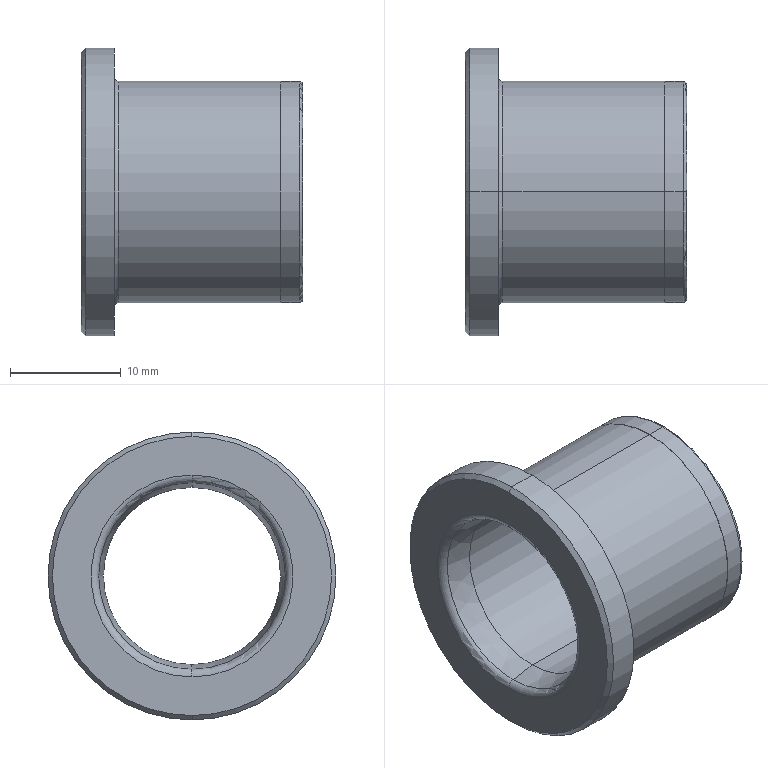Part | SolidWorks | features Revolution 1 | 1 solid | 24 faces | box 20 x 26 x 26 mm | volume 2854 mm3 | cylinder 8 | torus 8 | cone 4 | plane 4 | commonest cylinder face diameters 16 x2 19.96 x2 20 x2 26 x2
STEP:
#1=CARTESIAN_POINT('',(3.,0.,13.));
#2=VERTEX_POINT('',#1);
#3=CARTESIAN_POINT('',(3.,0.,-13.));
#4=VERTEX_POINT('',#3);
#5=CARTESIAN_POINT('',(3.,0.,0.));
#6=DIRECTION('',(-1.,0.,0.));
#7=DIRECTION('',(0.,0.,1.));
#8=AXIS2_PLACEMENT_3D('',#5,#6,#7);
#9=CIRCLE('',#8,13.);
#10=EDGE_CURVE('',#2,#4,#9,.T.);
#11=ORIENTED_EDGE('',*,*,#10,.T.);
#12=CARTESIAN_POINT('',(0.4,0.,-13.));
#13=VERTEX_POINT('',#12);
#14=CARTESIAN_POINT('',(20.,0.,-13.));
#15=DIRECTION('',(-1.,0.,0.));
#16=VECTOR('',#15,1000.);
#17=LINE('',#14,#16);
#18=EDGE_CURVE('',#4,#13,#17,.T.);
#19=ORIENTED_EDGE('',*,*,#18,.T.);
#20=CARTESIAN_POINT('',(0.4,0.,13.));
#21=VERTEX_POINT('',#20);
#22=CARTESIAN_POINT('',(0.4,0.,0.));
#23=DIRECTION('',(-1.,0.,0.));
#24=DIRECTION('',(0.,0.,1.));
#25=AXIS2_PLACEMENT_3D('',#22,#23,#24);
#26=CIRCLE('',#25,13.);
#27=EDGE_CURVE('',#21,#13,#26,.T.);
#28=ORIENTED_EDGE('',*,*,#27,.F.);
#29=CARTESIAN_POINT('',(20.,0.,13.));
#30=DIRECTION('',(-1.,0.,0.));
#31=VECTOR('',#30,1000.);
#32=LINE('',#29,#31);
#33=EDGE_CURVE('',#2,#21,#32,.T.);
#34=ORIENTED_EDGE('',*,*,#33,.F.);
#35=EDGE_LOOP('',(#11,#19,#28,#34));
#36=FACE_OUTER_BOUND('',#35,.T.);
#37=CARTESIAN_POINT('',(20.,0.,0.));
#38=DIRECTION('',(-1.,0.,0.));
#39=DIRECTION('',(0.,0.,1.));
#40=AXIS2_PLACEMENT_3D('',#37,#38,#39);
#41=CYLINDRICAL_SURFACE('',#40,13.);
#42=ADVANCED_FACE('',(#36),#41,.T.);
#43=CARTESIAN_POINT('',(3.,0.,-10.4));
#44=VERTEX_POINT('',#43);
#45=CARTESIAN_POINT('',(3.,0.,10.4));
#46=VERTEX_POINT('',#45);
#47=CARTESIAN_POINT('',(3.,0.,0.));
#48=DIRECTION('',(-1.,0.,0.));
#49=DIRECTION('',(0.,0.,1.));
#50=AXIS2_PLACEMENT_3D('',#47,#48,#49);
#51=CIRCLE('',#50,10.4);
#52=EDGE_CURVE('',#44,#46,#51,.T.);
#53=ORIENTED_EDGE('',*,*,#52,.F.);
#54=CARTESIAN_POINT('',(3.4,0.,-10.));
#55=VERTEX_POINT('',#54);
#56=CARTESIAN_POINT('',(3.4,0.,-10.4));
#57=DIRECTION('',(0.,1.,0.));
#58=DIRECTION('',(0.,0.,1.));
#59=AXIS2_PLACEMENT_3D('',#56,#57,#58);
#60=CIRCLE('',#59,0.4);
#61=EDGE_CURVE('',#44,#55,#60,.T.);
#62=ORIENTED_EDGE('',*,*,#61,.T.);
#63=CARTESIAN_POINT('',(3.4,0.,10.));
#64=VERTEX_POINT('',#63);
#65=CARTESIAN_POINT('',(3.4,0.,0.));
#66=DIRECTION('',(-1.,0.,0.));
#67=DIRECTION('',(0.,0.,1.));
#68=AXIS2_PLACEMENT_3D('',#65,#66,#67);
#69=CIRCLE('',#68,10.);
#70=EDGE_CURVE('',#55,#64,#69,.T.);
#71=ORIENTED_EDGE('',*,*,#70,.T.);
#72=CARTESIAN_POINT('',(3.4,0.,10.4));
#73=DIRECTION('',(0.,-1.,0.));
#74=DIRECTION('',(0.,0.,-1.));
#75=AXIS2_PLACEMENT_3D('',#72,#73,#74);
#76=CIRCLE('',#75,0.4);
#77=EDGE_CURVE('',#46,#64,#76,.T.);
#78=ORIENTED_EDGE('',*,*,#77,.F.);
#79=EDGE_LOOP('',(#53,#62,#71,#78));
#80=FACE_OUTER_BOUND('',#79,.T.);
#81=CARTESIAN_POINT('',(3.4,0.,0.));
#82=DIRECTION('',(-1.,0.,0.));
#83=DIRECTION('',(0.,0.,1.));
#84=AXIS2_PLACEMENT_3D('',#81,#82,#83);
#85=TOROIDAL_SURFACE('',#84,10.4,0.4);
#86=ADVANCED_FACE('',(#80),#85,.F.);
#87=CARTESIAN_POINT('',(18.,0.,10.));
#88=VERTEX_POINT('',#87);
#89=CARTESIAN_POINT('',(18.,0.,-10.));
#90=VERTEX_POINT('',#89);
#91=CARTESIAN_POINT('',(18.,0.,0.));
#92=DIRECTION('',(-1.,0.,0.));
#93=DIRECTION('',(0.,0.,1.));
#94=AXIS2_PLACEMENT_3D('',#91,#92,#93);
#95=CIRCLE('',#94,10.);
#96=EDGE_CURVE('',#88,#90,#95,.T.);
#97=ORIENTED_EDGE('',*,*,#96,.T.);
#98=CARTESIAN_POINT('',(20.,0.,-10.));
#99=DIRECTION('',(-1.,0.,0.));
#100=VECTOR('',#99,1000.);
#101=LINE('',#98,#100);
#102=EDGE_CURVE('',#90,#55,#101,.T.);
#103=ORIENTED_EDGE('',*,*,#102,.T.);
#104=CARTESIAN_POINT('',(3.4,0.,0.));
#105=DIRECTION('',(-1.,0.,0.));
#106=DIRECTION('',(0.,0.,1.));
#107=AXIS2_PLACEMENT_3D('',#104,#105,#106);
#108=CIRCLE('',#107,10.);
#109=EDGE_CURVE('',#64,#55,#108,.T.);
#110=ORIENTED_EDGE('',*,*,#109,.F.);
#111=CARTESIAN_POINT('',(20.,0.,10.));
#112=DIRECTION('',(-1.,0.,0.));
#113=VECTOR('',#112,1000.);
#114=LINE('',#111,#113);
#115=EDGE_CURVE('',#88,#64,#114,.T.);
#116=ORIENTED_EDGE('',*,*,#115,.F.);
#117=EDGE_LOOP('',(#97,#103,#110,#116));
#118=FACE_OUTER_BOUND('',#117,.T.);
#119=CARTESIAN_POINT('',(20.,0.,0.));
#120=DIRECTION('',(-1.,0.,0.));
#121=DIRECTION('',(0.,0.,1.));
#122=AXIS2_PLACEMENT_3D('',#119,#120,#121);
#123=CYLINDRICAL_SURFACE('',#122,10.);
#124=ADVANCED_FACE('',(#118),#123,.T.);
#125=CARTESIAN_POINT('',(19.7,0.,9.98));
#126=VERTEX_POINT('',#125);
#127=CARTESIAN_POINT('',(19.7,0.,-9.98));
#128=VERTEX_POINT('',#127);
#129=CARTESIAN_POINT('',(19.7,0.,0.));
#130=DIRECTION('',(-1.,0.,0.));
#131=DIRECTION('',(0.,0.,1.));
#132=AXIS2_PLACEMENT_3D('',#129,#130,#131);
#133=CIRCLE('',#132,9.98);
#134=EDGE_CURVE('',#126,#128,#133,.T.);
#135=ORIENTED_EDGE('',*,*,#134,.T.);
#136=CARTESIAN_POINT('',(18.,0.,-9.98));
#137=VERTEX_POINT('',#136);
#138=CARTESIAN_POINT('',(20.,0.,-9.98));
#139=DIRECTION('',(-1.,0.,0.));
#140=VECTOR('',#139,1000.);
#141=LINE('',#138,#140);
#142=EDGE_CURVE('',#128,#137,#141,.T.);
#143=ORIENTED_EDGE('',*,*,#142,.T.);
#144=CARTESIAN_POINT('',(18.,0.,9.98));
#145=VERTEX_POINT('',#144);
#146=CARTESIAN_POINT('',(18.,0.,0.));
#147=DIRECTION('',(-1.,0.,0.));
#148=DIRECTION('',(0.,0.,1.));
#149=AXIS2_PLACEMENT_3D('',#146,#147,#148);
#150=CIRCLE('',#149,9.98);
#151=EDGE_CURVE('',#145,#137,#150,.T.);
#152=ORIENTED_EDGE('',*,*,#151,.F.);
#153=CARTESIAN_POINT('',(20.,0.,9.98));
#154=DIRECTION('',(-1.,0.,0.));
#155=VECTOR('',#154,1000.);
#156=LINE('',#153,#155);
#157=EDGE_CURVE('',#126,#145,#156,.T.);
#158=ORIENTED_EDGE('',*,*,#157,.F.);
#159=EDGE_LOOP('',(#135,#143,#152,#158));
#160=FACE_OUTER_BOUND('',#159,.T.);
#161=CARTESIAN_POINT('',(20.,0.,0.));
#162=DIRECTION('',(-1.,0.,0.));
#163=DIRECTION('',(0.,0.,1.));
#164=AXIS2_PLACEMENT_3D('',#161,#162,#163);
#165=CYLINDRICAL_SURFACE('',#164,9.98);
#166=ADVANCED_FACE('',(#160),#165,.T.);
#167=CARTESIAN_POINT('',(20.,0.,9.68));
#168=VERTEX_POINT('',#167);
#169=CARTESIAN_POINT('',(20.,0.,-9.68));
#170=VERTEX_POINT('',#169);
#171=CARTESIAN_POINT('',(20.,0.,0.));
#172=DIRECTION('',(-1.,0.,0.));
#173=DIRECTION('',(0.,0.,1.));
#174=AXIS2_PLACEMENT_3D('',#171,#172,#173);
#175=CIRCLE('',#174,9.68);
#176=EDGE_CURVE('',#168,#170,#175,.T.);
#177=ORIENTED_EDGE('',*,*,#176,.T.);
#178=CARTESIAN_POINT('',(19.7,0.,-9.68));
#179=DIRECTION('',(0.,1.,0.));
#180=DIRECTION('',(0.,0.,1.));
#181=AXIS2_PLACEMENT_3D('',#178,#179,#180);
#182=CIRCLE('',#181,0.3);
#183=EDGE_CURVE('',#170,#128,#182,.T.);
#184=ORIENTED_EDGE('',*,*,#183,.T.);
#185=ORIENTED_EDGE('',*,*,#134,.F.);
#186=CARTESIAN_POINT('',(19.7,0.,9.68));
#187=DIRECTION('',(0.,-1.,0.));
#188=DIRECTION('',(0.,0.,-1.));
#189=AXIS2_PLACEMENT_3D('',#186,#187,#188);
#190=CIRCLE('',#189,0.3);
#191=EDGE_CURVE('',#168,#126,#190,.T.);
#192=ORIENTED_EDGE('',*,*,#191,.F.);
#193=EDGE_LOOP('',(#177,#184,#185,#192));
#194=FACE_OUTER_BOUND('',#193,.T.);
#195=CARTESIAN_POINT('',(19.7,0.,0.));
#196=DIRECTION('',(-1.,0.,0.));
#197=DIRECTION('',(0.,0.,1.));
#198=AXIS2_PLACEMENT_3D('',#195,#196,#197);
#199=TOROIDAL_SURFACE('',#198,9.68,0.3);
#200=ADVANCED_FACE('',(#194),#199,.T.);
#201=CARTESIAN_POINT('',(19.3,0.,8.));
#202=VERTEX_POINT('',#201);
#203=CARTESIAN_POINT('',(19.3,0.,-8.));
#204=VERTEX_POINT('',#203);
#205=CARTESIAN_POINT('',(19.3,0.,0.));
#206=DIRECTION('',(-1.,0.,0.));
#207=DIRECTION('',(0.,0.,1.));
#208=AXIS2_PLACEMENT_3D('',#205,#206,#207);
#209=CIRCLE('',#208,8.);
#210=EDGE_CURVE('',#202,#204,#209,.T.);
#211=ORIENTED_EDGE('',*,*,#210,.T.);
#212=CARTESIAN_POINT('',(20.,0.,-8.7));
#213=VERTEX_POINT('',#212);
#214=CARTESIAN_POINT('',(19.3,0.,-8.7));
#215=DIRECTION('',(0.,1.,0.));
#216=DIRECTION('',(0.,0.,1.));
#217=AXIS2_PLACEMENT_3D('',#214,#215,#216);
#218=CIRCLE('',#217,0.7);
#219=EDGE_CURVE('',#204,#213,#218,.T.);
#220=ORIENTED_EDGE('',*,*,#219,.T.);
#221=CARTESIAN_POINT('',(20.,0.,8.7));
#222=VERTEX_POINT('',#221);
#223=CARTESIAN_POINT('',(20.,0.,0.));
#224=DIRECTION('',(-1.,0.,0.));
#225=DIRECTION('',(0.,0.,1.));
#226=AXIS2_PLACEMENT_3D('',#223,#224,#225);
#227=CIRCLE('',#226,8.7);
#228=EDGE_CURVE('',#222,#213,#227,.T.);
#229=ORIENTED_EDGE('',*,*,#228,.F.);
#230=CARTESIAN_POINT('',(19.3,0.,8.7));
#231=DIRECTION('',(0.,-1.,0.));
#232=DIRECTION('',(0.,0.,-1.));
#233=AXIS2_PLACEMENT_3D('',#230,#231,#232);
#234=CIRCLE('',#233,0.7);
#235=EDGE_CURVE('',#202,#222,#234,.T.);
#236=ORIENTED_EDGE('',*,*,#235,.F.);
#237=EDGE_LOOP('',(#211,#220,#229,#236));
#238=FACE_OUTER_BOUND('',#237,.T.);
#239=CARTESIAN_POINT('',(19.3,0.,0.));
#240=DIRECTION('',(-1.,0.,0.));
#241=DIRECTION('',(0.,0.,1.));
#242=AXIS2_PLACEMENT_3D('',#239,#240,#241);
#243=TOROIDAL_SURFACE('',#242,8.7,0.7);
#244=ADVANCED_FACE('',(#238),#243,.T.);
#245=CARTESIAN_POINT('',(19.3,0.,0.));
#246=DIRECTION('',(-1.,0.,0.));
#247=DIRECTION('',(0.,0.,1.));
#248=AXIS2_PLACEMENT_3D('',#245,#246,#247);
#249=CIRCLE('',#248,8.);
#250=EDGE_CURVE('',#204,#202,#249,.T.);
#251=ORIENTED_EDGE('',*,*,#250,.F.);
#252=CARTESIAN_POINT('',(3.,0.,-8.));
#253=VERTEX_POINT('',#252);
#254=CARTESIAN_POINT('',(20.,0.,-8.));
#255=DIRECTION('',(-1.,0.,0.));
#256=VECTOR('',#255,1000.);
#257=LINE('',#254,#256);
#258=EDGE_CURVE('',#204,#253,#257,.T.);
#259=ORIENTED_EDGE('',*,*,#258,.T.);
#260=CARTESIAN_POINT('',(3.,0.,8.));
#261=VERTEX_POINT('',#260);
#262=CARTESIAN_POINT('',(3.,0.,0.));
#263=DIRECTION('',(-1.,0.,0.));
#264=DIRECTION('',(0.,0.,1.));
#265=AXIS2_PLACEMENT_3D('',#262,#263,#264);
#266=CIRCLE('',#265,8.);
#267=EDGE_CURVE('',#253,#261,#266,.T.);
#268=ORIENTED_EDGE('',*,*,#267,.T.);
#269=CARTESIAN_POINT('',(20.,0.,8.));
#270=DIRECTION('',(-1.,0.,0.));
#271=VECTOR('',#270,1000.);
#272=LINE('',#269,#271);
#273=EDGE_CURVE('',#202,#261,#272,.T.);
#274=ORIENTED_EDGE('',*,*,#273,.F.);
#275=EDGE_LOOP('',(#251,#259,#268,#274));
#276=FACE_OUTER_BOUND('',#275,.T.);
#277=CARTESIAN_POINT('',(20.,0.,0.));
#278=DIRECTION('',(-1.,0.,0.));
#279=DIRECTION('',(0.,0.,1.));
#280=AXIS2_PLACEMENT_3D('',#277,#278,#279);
#281=CYLINDRICAL_SURFACE('',#280,8.);
#282=ADVANCED_FACE('',(#276),#281,.F.);
#283=ORIENTED_EDGE('',*,*,#267,.F.);
#284=CARTESIAN_POINT('',(0.5784,0.,-8.427));
#285=VERTEX_POINT('',#284);
#286=CARTESIAN_POINT('',(0.5784,0.,-8.427));
#287=DIRECTION('',(-0.9848,0.,-0.1736));
#288=VECTOR('',#287,1000.);
#289=LINE('',#286,#288);
#290=EDGE_CURVE('',#253,#285,#289,.T.);
#291=ORIENTED_EDGE('',*,*,#290,.T.);
#292=CARTESIAN_POINT('',(0.5784,0.,8.427));
#293=VERTEX_POINT('',#292);
#294=CARTESIAN_POINT('',(0.5784,0.,0.));
#295=DIRECTION('',(-1.,0.,0.));
#296=DIRECTION('',(0.,0.,1.));
#297=AXIS2_PLACEMENT_3D('',#294,#295,#296);
#298=CIRCLE('',#297,8.427);
#299=EDGE_CURVE('',#285,#293,#298,.T.);
#300=ORIENTED_EDGE('',*,*,#299,.T.);
#301=CARTESIAN_POINT('',(0.5784,0.,8.427));
#302=DIRECTION('',(-0.9848,0.,0.1736));
#303=VECTOR('',#302,1000.);
#304=LINE('',#301,#303);
#305=EDGE_CURVE('',#261,#293,#304,.T.);
#306=ORIENTED_EDGE('',*,*,#305,.F.);
#307=EDGE_LOOP('',(#283,#291,#300,#306));
#308=FACE_OUTER_BOUND('',#307,.T.);
#309=CARTESIAN_POINT('',(0.5784,0.,0.));
#310=DIRECTION('',(-1.,0.,0.));
#311=DIRECTION('',(0.,0.,1.));
#312=AXIS2_PLACEMENT_3D('',#309,#310,#311);
#313=CONICAL_SURFACE('',#312,8.427,0.1745);
#314=ADVANCED_FACE('',(#308),#313,.F.);
#315=CARTESIAN_POINT('',(0.,0.,9.116));
#316=VERTEX_POINT('',#315);
#317=CARTESIAN_POINT('',(0.,0.,-9.116));
#318=VERTEX_POINT('',#317);
#319=CARTESIAN_POINT('',(0.,0.,0.));
#320=DIRECTION('',(-1.,0.,0.));
#321=DIRECTION('',(0.,0.,1.));
#322=AXIS2_PLACEMENT_3D('',#319,#320,#321);
#323=CIRCLE('',#322,9.116);
#324=EDGE_CURVE('',#316,#318,#323,.T.);
#325=ORIENTED_EDGE('',*,*,#324,.T.);
#326=CARTESIAN_POINT('',(0.7,0.,-9.116));
#327=DIRECTION('',(0.,1.,0.));
#328=DIRECTION('',(0.,0.,1.));
#329=AXIS2_PLACEMENT_3D('',#326,#327,#328);
#330=CIRCLE('',#329,0.7);
#331=EDGE_CURVE('',#318,#285,#330,.T.);
#332=ORIENTED_EDGE('',*,*,#331,.T.);
#333=CARTESIAN_POINT('',(0.5784,0.,0.));
#334=DIRECTION('',(-1.,0.,0.));
#335=DIRECTION('',(0.,0.,1.));
#336=AXIS2_PLACEMENT_3D('',#333,#334,#335);
#337=CIRCLE('',#336,8.427);
#338=EDGE_CURVE('',#293,#285,#337,.T.);
#339=ORIENTED_EDGE('',*,*,#338,.F.);
#340=CARTESIAN_POINT('',(0.7,0.,9.116));
#341=DIRECTION('',(0.,-1.,0.));
#342=DIRECTION('',(0.,0.,-1.));
#343=AXIS2_PLACEMENT_3D('',#340,#341,#342);
#344=CIRCLE('',#343,0.7);
#345=EDGE_CURVE('',#316,#293,#344,.T.);
#346=ORIENTED_EDGE('',*,*,#345,.F.);
#347=EDGE_LOOP('',(#325,#332,#339,#346));
#348=FACE_OUTER_BOUND('',#347,.T.);
#349=CARTESIAN_POINT('',(0.7,0.,0.));
#350=DIRECTION('',(-1.,0.,0.));
#351=DIRECTION('',(0.,0.,1.));
#352=AXIS2_PLACEMENT_3D('',#349,#350,#351);
#353=TOROIDAL_SURFACE('',#352,9.116,0.7);
#354=ADVANCED_FACE('',(#348),#353,.T.);
#355=CARTESIAN_POINT('',(0.,0.,12.6));
#356=VERTEX_POINT('',#355);
#357=CARTESIAN_POINT('',(0.,0.,-12.6));
#358=VERTEX_POINT('',#357);
#359=CARTESIAN_POINT('',(0.,0.,0.));
#360=DIRECTION('',(-1.,0.,0.));
#361=DIRECTION('',(0.,0.,1.));
#362=AXIS2_PLACEMENT_3D('',#359,#360,#361);
#363=CIRCLE('',#362,12.6);
#364=EDGE_CURVE('',#356,#358,#363,.T.);
#365=ORIENTED_EDGE('',*,*,#364,.F.);
#366=CARTESIAN_POINT('',(0.4,0.,13.));
#367=DIRECTION('',(0.7071,0.,0.7071));
#368=VECTOR('',#367,1000.);
#369=LINE('',#366,#368);
#370=EDGE_CURVE('',#356,#21,#369,.T.);
#371=ORIENTED_EDGE('',*,*,#370,.T.);
#372=ORIENTED_EDGE('',*,*,#27,.T.);
#373=CARTESIAN_POINT('',(0.4,0.,-13.));
#374=DIRECTION('',(0.7071,0.,-0.7071));
#375=VECTOR('',#374,1000.);
#376=LINE('',#373,#375);
#377=EDGE_CURVE('',#358,#13,#376,.T.);
#378=ORIENTED_EDGE('',*,*,#377,.F.);
#379=EDGE_LOOP('',(#365,#371,#372,#378));
#380=FACE_OUTER_BOUND('',#379,.T.);
#381=CARTESIAN_POINT('',(0.4,0.,0.));
#382=DIRECTION('',(1.,0.,0.));
#383=DIRECTION('',(0.,0.,-1.));
#384=AXIS2_PLACEMENT_3D('',#381,#382,#383);
#385=CONICAL_SURFACE('',#384,13.,0.7854);
#386=ADVANCED_FACE('',(#380),#385,.T.);
#387=ORIENTED_EDGE('',*,*,#370,.F.);
#388=CARTESIAN_POINT('',(0.,0.,0.));
#389=DIRECTION('',(-1.,0.,0.));
#390=DIRECTION('',(0.,0.,1.));
#391=AXIS2_PLACEMENT_3D('',#388,#389,#390);
#392=CIRCLE('',#391,12.6);
#393=EDGE_CURVE('',#358,#356,#392,.T.);
#394=ORIENTED_EDGE('',*,*,#393,.F.);
#395=ORIENTED_EDGE('',*,*,#377,.T.);
#396=CARTESIAN_POINT('',(0.4,0.,0.));
#397=DIRECTION('',(-1.,0.,0.));
#398=DIRECTION('',(0.,0.,1.));
#399=AXIS2_PLACEMENT_3D('',#396,#397,#398);
#400=CIRCLE('',#399,13.);
#401=EDGE_CURVE('',#13,#21,#400,.T.);
#402=ORIENTED_EDGE('',*,*,#401,.T.);
#403=EDGE_LOOP('',(#387,#394,#395,#402));
#404=FACE_OUTER_BOUND('',#403,.T.);
#405=CARTESIAN_POINT('',(0.4,0.,0.));
#406=DIRECTION('',(1.,0.,0.));
#407=DIRECTION('',(0.,0.,-1.));
#408=AXIS2_PLACEMENT_3D('',#405,#406,#407);
#409=CONICAL_SURFACE('',#408,13.,0.7854);
#410=ADVANCED_FACE('',(#404),#409,.T.);
#411=ORIENTED_EDGE('',*,*,#324,.F.);
#412=CARTESIAN_POINT('',(0.,0.,0.));
#413=DIRECTION('',(-1.,0.,0.));
#414=DIRECTION('',(0.,0.,1.));
#415=AXIS2_PLACEMENT_3D('',#412,#413,#414);
#416=CIRCLE('',#415,9.116);
#417=EDGE_CURVE('',#318,#316,#416,.T.);
#418=ORIENTED_EDGE('',*,*,#417,.F.);
#419=EDGE_LOOP('',(#411,#418));
#420=FACE_BOUND('',#419,.T.);
#421=ORIENTED_EDGE('',*,*,#393,.T.);
#422=ORIENTED_EDGE('',*,*,#364,.T.);
#423=EDGE_LOOP('',(#421,#422));
#424=FACE_OUTER_BOUND('',#423,.T.);
#425=CARTESIAN_POINT('',(0.,12.6,0.));
#426=DIRECTION('',(1.,0.,0.));
#427=DIRECTION('',(0.,0.,-1.));
#428=AXIS2_PLACEMENT_3D('',#425,#426,#427);
#429=PLANE('',#428);
#430=ADVANCED_FACE('',(#420,#424),#429,.F.);
#431=ORIENTED_EDGE('',*,*,#331,.F.);
#432=ORIENTED_EDGE('',*,*,#417,.T.);
#433=ORIENTED_EDGE('',*,*,#345,.T.);
#434=ORIENTED_EDGE('',*,*,#299,.F.);
#435=EDGE_LOOP('',(#431,#432,#433,#434));
#436=FACE_OUTER_BOUND('',#435,.T.);
#437=CARTESIAN_POINT('',(0.7,0.,0.));
#438=DIRECTION('',(-1.,0.,0.));
#439=DIRECTION('',(0.,0.,1.));
#440=AXIS2_PLACEMENT_3D('',#437,#438,#439);
#441=TOROIDAL_SURFACE('',#440,9.116,0.7);
#442=ADVANCED_FACE('',(#436),#441,.T.);
#443=ORIENTED_EDGE('',*,*,#290,.F.);
#444=CARTESIAN_POINT('',(3.,0.,0.));
#445=DIRECTION('',(-1.,0.,0.));
#446=DIRECTION('',(0.,0.,1.));
#447=AXIS2_PLACEMENT_3D('',#444,#445,#446);
#448=CIRCLE('',#447,8.);
#449=EDGE_CURVE('',#261,#253,#448,.T.);
#450=ORIENTED_EDGE('',*,*,#449,.F.);
#451=ORIENTED_EDGE('',*,*,#305,.T.);
#452=ORIENTED_EDGE('',*,*,#338,.T.);
#453=EDGE_LOOP('',(#443,#450,#451,#452));
#454=FACE_OUTER_BOUND('',#453,.T.);
#455=CARTESIAN_POINT('',(0.5784,0.,0.));
#456=DIRECTION('',(-1.,0.,0.));
#457=DIRECTION('',(0.,0.,1.));
#458=AXIS2_PLACEMENT_3D('',#455,#456,#457);
#459=CONICAL_SURFACE('',#458,8.427,0.1745);
#460=ADVANCED_FACE('',(#454),#459,.F.);
#461=ORIENTED_EDGE('',*,*,#258,.F.);
#462=ORIENTED_EDGE('',*,*,#210,.F.);
#463=ORIENTED_EDGE('',*,*,#273,.T.);
#464=ORIENTED_EDGE('',*,*,#449,.T.);
#465=EDGE_LOOP('',(#461,#462,#463,#464));
#466=FACE_OUTER_BOUND('',#465,.T.);
#467=CARTESIAN_POINT('',(20.,0.,0.));
#468=DIRECTION('',(-1.,0.,0.));
#469=DIRECTION('',(0.,0.,1.));
#470=AXIS2_PLACEMENT_3D('',#467,#468,#469);
#471=CYLINDRICAL_SURFACE('',#470,8.);
#472=ADVANCED_FACE('',(#466),#471,.F.);
#473=ORIENTED_EDGE('',*,*,#219,.F.);
#474=ORIENTED_EDGE('',*,*,#250,.T.);
#475=ORIENTED_EDGE('',*,*,#235,.T.);
#476=CARTESIAN_POINT('',(20.,0.,0.));
#477=DIRECTION('',(-1.,0.,0.));
#478=DIRECTION('',(0.,0.,1.));
#479=AXIS2_PLACEMENT_3D('',#476,#477,#478);
#480=CIRCLE('',#479,8.7);
#481=EDGE_CURVE('',#213,#222,#480,.T.);
#482=ORIENTED_EDGE('',*,*,#481,.F.);
#483=EDGE_LOOP('',(#473,#474,#475,#482));
#484=FACE_OUTER_BOUND('',#483,.T.);
#485=CARTESIAN_POINT('',(19.3,0.,0.));
#486=DIRECTION('',(-1.,0.,0.));
#487=DIRECTION('',(0.,0.,1.));
#488=AXIS2_PLACEMENT_3D('',#485,#486,#487);
#489=TOROIDAL_SURFACE('',#488,8.7,0.7);
#490=ADVANCED_FACE('',(#484),#489,.T.);
#491=ORIENTED_EDGE('',*,*,#176,.F.);
#492=CARTESIAN_POINT('',(20.,0.,0.));
#493=DIRECTION('',(-1.,0.,0.));
#494=DIRECTION('',(0.,0.,1.));
#495=AXIS2_PLACEMENT_3D('',#492,#493,#494);
#496=CIRCLE('',#495,9.68);
#497=EDGE_CURVE('',#170,#168,#496,.T.);
#498=ORIENTED_EDGE('',*,*,#497,.F.);
#499=EDGE_LOOP('',(#491,#498));
#500=FACE_OUTER_BOUND('',#499,.T.);
#501=ORIENTED_EDGE('',*,*,#228,.T.);
#502=ORIENTED_EDGE('',*,*,#481,.T.);
#503=EDGE_LOOP('',(#501,#502));
#504=FACE_BOUND('',#503,.T.);
#505=CARTESIAN_POINT('',(20.,8.7,0.));
#506=DIRECTION('',(-1.,0.,0.));
#507=DIRECTION('',(0.,0.,1.));
#508=AXIS2_PLACEMENT_3D('',#505,#506,#507);
#509=PLANE('',#508);
#510=ADVANCED_FACE('',(#500,#504),#509,.F.);
#511=ORIENTED_EDGE('',*,*,#183,.F.);
#512=ORIENTED_EDGE('',*,*,#497,.T.);
#513=ORIENTED_EDGE('',*,*,#191,.T.);
#514=CARTESIAN_POINT('',(19.7,0.,0.));
#515=DIRECTION('',(-1.,0.,0.));
#516=DIRECTION('',(0.,0.,1.));
#517=AXIS2_PLACEMENT_3D('',#514,#515,#516);
#518=CIRCLE('',#517,9.98);
#519=EDGE_CURVE('',#128,#126,#518,.T.);
#520=ORIENTED_EDGE('',*,*,#519,.F.);
#521=EDGE_LOOP('',(#511,#512,#513,#520));
#522=FACE_OUTER_BOUND('',#521,.T.);
#523=CARTESIAN_POINT('',(19.7,0.,0.));
#524=DIRECTION('',(-1.,0.,0.));
#525=DIRECTION('',(0.,0.,1.));
#526=AXIS2_PLACEMENT_3D('',#523,#524,#525);
#527=TOROIDAL_SURFACE('',#526,9.68,0.3);
#528=ADVANCED_FACE('',(#522),#527,.T.);
#529=ORIENTED_EDGE('',*,*,#142,.F.);
#530=ORIENTED_EDGE('',*,*,#519,.T.);
#531=ORIENTED_EDGE('',*,*,#157,.T.);
#532=CARTESIAN_POINT('',(18.,0.,0.));
#533=DIRECTION('',(-1.,0.,0.));
#534=DIRECTION('',(0.,0.,1.));
#535=AXIS2_PLACEMENT_3D('',#532,#533,#534);
#536=CIRCLE('',#535,9.98);
#537=EDGE_CURVE('',#137,#145,#536,.T.);
#538=ORIENTED_EDGE('',*,*,#537,.F.);
#539=EDGE_LOOP('',(#529,#530,#531,#538));
#540=FACE_OUTER_BOUND('',#539,.T.);
#541=CARTESIAN_POINT('',(20.,0.,0.));
#542=DIRECTION('',(-1.,0.,0.));
#543=DIRECTION('',(0.,0.,1.));
#544=AXIS2_PLACEMENT_3D('',#541,#542,#543);
#545=CYLINDRICAL_SURFACE('',#544,9.98);
#546=ADVANCED_FACE('',(#540),#545,.T.);
#547=ORIENTED_EDGE('',*,*,#96,.F.);
#548=CARTESIAN_POINT('',(18.,0.,0.));
#549=DIRECTION('',(-1.,0.,0.));
#550=DIRECTION('',(0.,0.,1.));
#551=AXIS2_PLACEMENT_3D('',#548,#549,#550);
#552=CIRCLE('',#551,10.);
#553=EDGE_CURVE('',#90,#88,#552,.T.);
#554=ORIENTED_EDGE('',*,*,#553,.F.);
#555=EDGE_LOOP('',(#547,#554));
#556=FACE_OUTER_BOUND('',#555,.T.);
#557=ORIENTED_EDGE('',*,*,#151,.T.);
#558=ORIENTED_EDGE('',*,*,#537,.T.);
#559=EDGE_LOOP('',(#557,#558));
#560=FACE_BOUND('',#559,.T.);
#561=CARTESIAN_POINT('',(18.,9.98,0.));
#562=DIRECTION('',(-1.,0.,0.));
#563=DIRECTION('',(0.,0.,1.));
#564=AXIS2_PLACEMENT_3D('',#561,#562,#563);
#565=PLANE('',#564);
#566=ADVANCED_FACE('',(#556,#560),#565,.F.);
#567=ORIENTED_EDGE('',*,*,#102,.F.);
#568=ORIENTED_EDGE('',*,*,#553,.T.);
#569=ORIENTED_EDGE('',*,*,#115,.T.);
#570=ORIENTED_EDGE('',*,*,#70,.F.);
#571=EDGE_LOOP('',(#567,#568,#569,#570));
#572=FACE_OUTER_BOUND('',#571,.T.);
#573=CARTESIAN_POINT('',(20.,0.,0.));
#574=DIRECTION('',(-1.,0.,0.));
#575=DIRECTION('',(0.,0.,1.));
#576=AXIS2_PLACEMENT_3D('',#573,#574,#575);
#577=CYLINDRICAL_SURFACE('',#576,10.);
#578=ADVANCED_FACE('',(#572),#577,.T.);
#579=ORIENTED_EDGE('',*,*,#61,.F.);
#580=CARTESIAN_POINT('',(3.,0.,0.));
#581=DIRECTION('',(-1.,0.,0.));
#582=DIRECTION('',(0.,0.,1.));
#583=AXIS2_PLACEMENT_3D('',#580,#581,#582);
#584=CIRCLE('',#583,10.4);
#585=EDGE_CURVE('',#46,#44,#584,.T.);
#586=ORIENTED_EDGE('',*,*,#585,.F.);
#587=ORIENTED_EDGE('',*,*,#77,.T.);
#588=ORIENTED_EDGE('',*,*,#109,.T.);
#589=EDGE_LOOP('',(#579,#586,#587,#588));
#590=FACE_OUTER_BOUND('',#589,.T.);
#591=CARTESIAN_POINT('',(3.4,0.,0.));
#592=DIRECTION('',(-1.,0.,0.));
#593=DIRECTION('',(0.,0.,1.));
#594=AXIS2_PLACEMENT_3D('',#591,#592,#593);
#595=TOROIDAL_SURFACE('',#594,10.4,0.4);
#596=ADVANCED_FACE('',(#590),#595,.F.);
#597=ORIENTED_EDGE('',*,*,#10,.F.);
#598=CARTESIAN_POINT('',(3.,0.,0.));
#599=DIRECTION('',(-1.,0.,0.));
#600=DIRECTION('',(0.,0.,1.));
#601=AXIS2_PLACEMENT_3D('',#598,#599,#600);
#602=CIRCLE('',#601,13.);
#603=EDGE_CURVE('',#4,#2,#602,.T.);
#604=ORIENTED_EDGE('',*,*,#603,.F.);
#605=EDGE_LOOP('',(#597,#604));
#606=FACE_OUTER_BOUND('',#605,.T.);
#607=ORIENTED_EDGE('',*,*,#585,.T.);
#608=ORIENTED_EDGE('',*,*,#52,.T.);
#609=EDGE_LOOP('',(#607,#608));
#610=FACE_BOUND('',#609,.T.);
#611=CARTESIAN_POINT('',(3.,10.4,0.));
#612=DIRECTION('',(-1.,0.,0.));
#613=DIRECTION('',(0.,0.,1.));
#614=AXIS2_PLACEMENT_3D('',#611,#612,#613);
#615=PLANE('',#614);
#616=ADVANCED_FACE('',(#606,#610),#615,.F.);
#617=ORIENTED_EDGE('',*,*,#18,.F.);
#618=ORIENTED_EDGE('',*,*,#603,.T.);
#619=ORIENTED_EDGE('',*,*,#33,.T.);
#620=ORIENTED_EDGE('',*,*,#401,.F.);
#621=EDGE_LOOP('',(#617,#618,#619,#620));
#622=FACE_OUTER_BOUND('',#621,.T.);
#623=CARTESIAN_POINT('',(20.,0.,0.));
#624=DIRECTION('',(-1.,0.,0.));
#625=DIRECTION('',(0.,0.,1.));
#626=AXIS2_PLACEMENT_3D('',#623,#624,#625);
#627=CYLINDRICAL_SURFACE('',#626,13.);
#628=ADVANCED_FACE('',(#622),#627,.T.);
#629=CLOSED_SHELL('',(#42,#86,#124,#166,#200,#244,#282,#314,#354,#386,#410,#430,#442,#460,#472,#490,#510,#528,#546,#566,#578,#596,#616,#628));
#630=MANIFOLD_SOLID_BREP('',#629);
#631=CARTESIAN_POINT('',(0.,0.,0.));
#632=DIRECTION('',(0.,0.,1.));
#633=DIRECTION('',(1.,0.,0.));
#634=AXIS2_PLACEMENT_3D('',#631,#632,#633);
#635=(LENGTH_UNIT()NAMED_UNIT(*)SI_UNIT(.MILLI.,.METRE.));
#636=UNCERTAINTY_MEASURE_WITH_UNIT(LENGTH_MEASURE(0.00001),#635,'','');
#637=(NAMED_UNIT(*)PLANE_ANGLE_UNIT()SI_UNIT($,.RADIAN.));
#638=(NAMED_UNIT(*)SI_UNIT($,.STERADIAN.)SOLID_ANGLE_UNIT());
#639=(GEOMETRIC_REPRESENTATION_CONTEXT(3)GLOBAL_UNCERTAINTY_ASSIGNED_CONTEXT((#636))GLOBAL_UNIT_ASSIGNED_CONTEXT((#635,#637,#638))REPRESENTATION_CONTEXT('',''));
#640=ADVANCED_BREP_SHAPE_REPRESENTATION('',(#630,#634),#639);